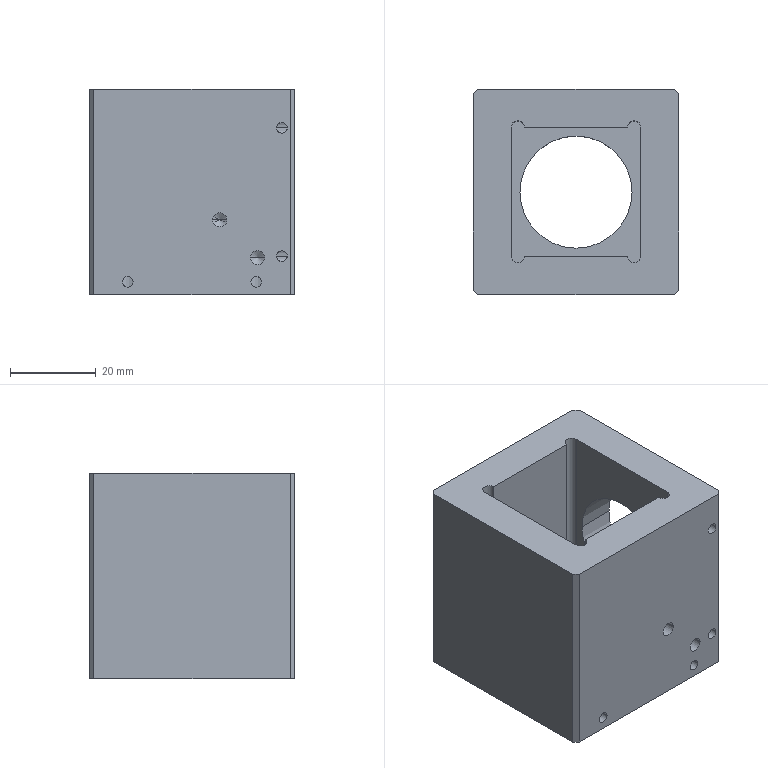NC program | NX | posted with a generic post | part box 48 x 48 x 48 mm
Whole program:
N10 G17 G21 G94 G90
(DRILLING_COPY_1_COPY_COPY , TOOL : D6A45)
N12 T01 M6
N14 G54
N16 G17 G0 G90 X-21. Y-15. B0. C0. S5000 M3
N18 G43 Z30. H1
N20 G94 G81 G98 Z-1. F350. R3.
N22 X-6.5 Y6.5
N24 X-15.339 Y15.339
N26 X-21. Y15.
N28 X-15. Y21.
N30 X15.
N32 G80
N34 G0 X15. Y21. Z30.
N36 M5
(DRILLING_COPY_1_COPY_1_1_COPY_1_1_COPY , TOOL : 3.3ZT)
N38 T03 M6
N40 G54
N42 G17 G0 G90 X-6.5 Y6.5 B0. C0. S2000 M3
N44 G43 Z30. H3
N46 G94 G83 G98 Z-6.991 F200. Q2. R3.
N48 X-15.339 Y15.339
N50 G80
N52 G0 X-15.339 Y15.339 Z30.
N54 M5
(PLANAR_MILL_COPY_COPY_COPY_COPY_COPY_COPY_1_COPY_1_COPY_COPY_COPY_COPY , TOOL )
N56 T01 M6
N58 G54
N60 G17 G0 G90 X14.756 Y21.373 B0. C0. S9500 M3
N62 G43 Z30. H1
N64 Z0.5
N66 G94 G1 X14.55 Y21.167 Z0.422 F1250.
N68 Y20.833 Z0.332
N70 X14.833 Y20.55 Z0.225
N72 X15.167 Z0.136
N74 X15.45 Y20.833 Z0.028
N76 Y21.167 Z-0.061
N78 X15.167 Y21.45 Z-0.168
N80 X14.833 Z-0.258
N82 X14.55 Y21.167 Z-0.365
N84 Y20.833 Z-0.455
N86 X14.833 Y20.55 Z-0.562
N88 X15.167 Z-0.651
N90 X15.45 Y20.833 Z-0.759
N92 Y21.167 Z-0.848
N94 X15.167 Y21.45 Z-0.955
N96 X15. Z-1.
N98 G3 X14.55 Y21. R0.45
N100 X15. Y21.45 R-0.45
N102 X14.75 Y21.383 R0.5
N104 G1 Z0.5
N106 G0 Z30.
N108 X-15.244 Y21.373
N110 Z0.5
N112 G1 X-15.45 Y21.167 Z0.422
N114 Y20.833 Z0.332
N116 X-15.167 Y20.55 Z0.225
N118 X-14.833 Z0.136
N120 X-14.55 Y20.833 Z0.028
N122 Y21.167 Z-0.061
N124 X-14.833 Y21.45 Z-0.168
N126 X-15.167 Z-0.258
N128 X-15.45 Y21.167 Z-0.365
N130 Y20.833 Z-0.455
N132 X-15.167 Y20.55 Z-0.562
N134 X-14.833 Z-0.651
N136 X-14.55 Y20.833 Z-0.759
N138 Y21.167 Z-0.848
N140 X-14.833 Y21.45 Z-0.955
N142 X-15. Z-1.
N144 G3 X-15.45 Y21. R0.45
N146 X-15. Y21.45 R-0.45
N148 X-15.25 Y21.383 R0.5
N150 G1 Z0.5
N152 G0 Z30.
N154 X-21.373 Y14.756
N156 Z0.5
N158 G1 X-21.167 Y14.55 Z0.422
N160 X-20.833 Z0.332
N162 X-20.55 Y14.833 Z0.225
N164 Y15.167 Z0.136
N166 X-20.833 Y15.45 Z0.028
N168 X-21.167 Z-0.061
N170 X-21.45 Y15.167 Z-0.168
N172 Y14.833 Z-0.258
N174 X-21.167 Y14.55 Z-0.365
N176 X-20.833 Z-0.455
N178 X-20.55 Y14.833 Z-0.562
N180 Y15.167 Z-0.651
N182 X-20.833 Y15.45 Z-0.759
N184 X-21.167 Z-0.848
N186 X-21.45 Y15.167 Z-0.955
N188 Y15. Z-1.
N190 G3 X-21. Y14.55 R0.45
N192 X-21.45 Y15. R-0.45
N194 X-21.383 Y14.75 R0.5
N196 G1 Z0.5
N198 G0 Z30.
N200 X-16.189 Y15.471
N202 Z0.5
N204 G1 Y15.111 Z0.404
N206 X-15.961 Y14.717 Z0.282
N208 X-15.567 Y14.489 Z0.16
N210 X-15.111 Z0.037
N212 X-14.717 Y14.717 Z-0.085
N214 X-14.489 Y15.111 Z-0.207
N216 Y15.567 Z-0.329
N218 X-14.717 Y15.961 Z-0.451
N220 X-15.111 Y16.189 Z-0.573
N222 X-15.567 Z-0.695
N224 X-15.961 Y15.961 Z-0.817
N226 X-16.189 Y15.567 Z-0.939
N228 Y15.339 Z-1.
N230 G3 X-15.339 Y14.489 R0.85
N232 X-16.189 Y15.339 R-0.85
N234 X-15.939 Y14.906 R0.5
N236 G1 Z0.5
N238 G0 Z30.
N240 X-7.35 Y6.632
N242 Z0.5
N244 G1 Y6.272 Z0.404
N246 X-7.122 Y5.878 Z0.282
N248 X-6.728 Y5.65 Z0.16
N250 X-6.272 Z0.037
N252 X-5.878 Y5.878 Z-0.085
N254 X-5.65 Y6.272 Z-0.207
N256 Y6.728 Z-0.329
N258 X-5.878 Y7.122 Z-0.451
N260 X-6.272 Y7.35 Z-0.573
N262 X-6.728 Z-0.695
N264 X-7.122 Y7.122 Z-0.817
N266 X-7.35 Y6.728 Z-0.939
N268 Y6.5 Z-1.
N270 G3 X-6.5 Y5.65 R0.85
N272 X-7.35 Y6.5 R-0.85
N274 X-7.1 Y6.067 R0.5
N276 G1 Z0.5
N278 G0 Z30.
N280 X-21.373 Y-15.244
N282 Z0.5
N284 G1 X-21.167 Y-15.45 Z0.422
N286 X-20.833 Z0.332
N288 X-20.55 Y-15.167 Z0.225
N290 Y-14.833 Z0.136
N292 X-20.833 Y-14.55 Z0.028
N294 X-21.167 Z-0.061
N296 X-21.45 Y-14.833 Z-0.168
N298 Y-15.167 Z-0.258
N300 X-21.167 Y-15.45 Z-0.365
N302 X-20.833 Z-0.455
N304 X-20.55 Y-15.167 Z-0.562
N306 Y-14.833 Z-0.651
N308 X-20.833 Y-14.55 Z-0.759
N310 X-21.167 Z-0.848
N312 X-21.45 Y-14.833 Z-0.955
N314 Y-15. Z-1.
N316 G3 X-21. Y-15.45 R0.45
N318 X-21.45 Y-15. R-0.45
N320 X-21.383 Y-15.25 R0.5
N322 G1 Z0.5
N324 G0 Z30.
N326 M5
N328 M2